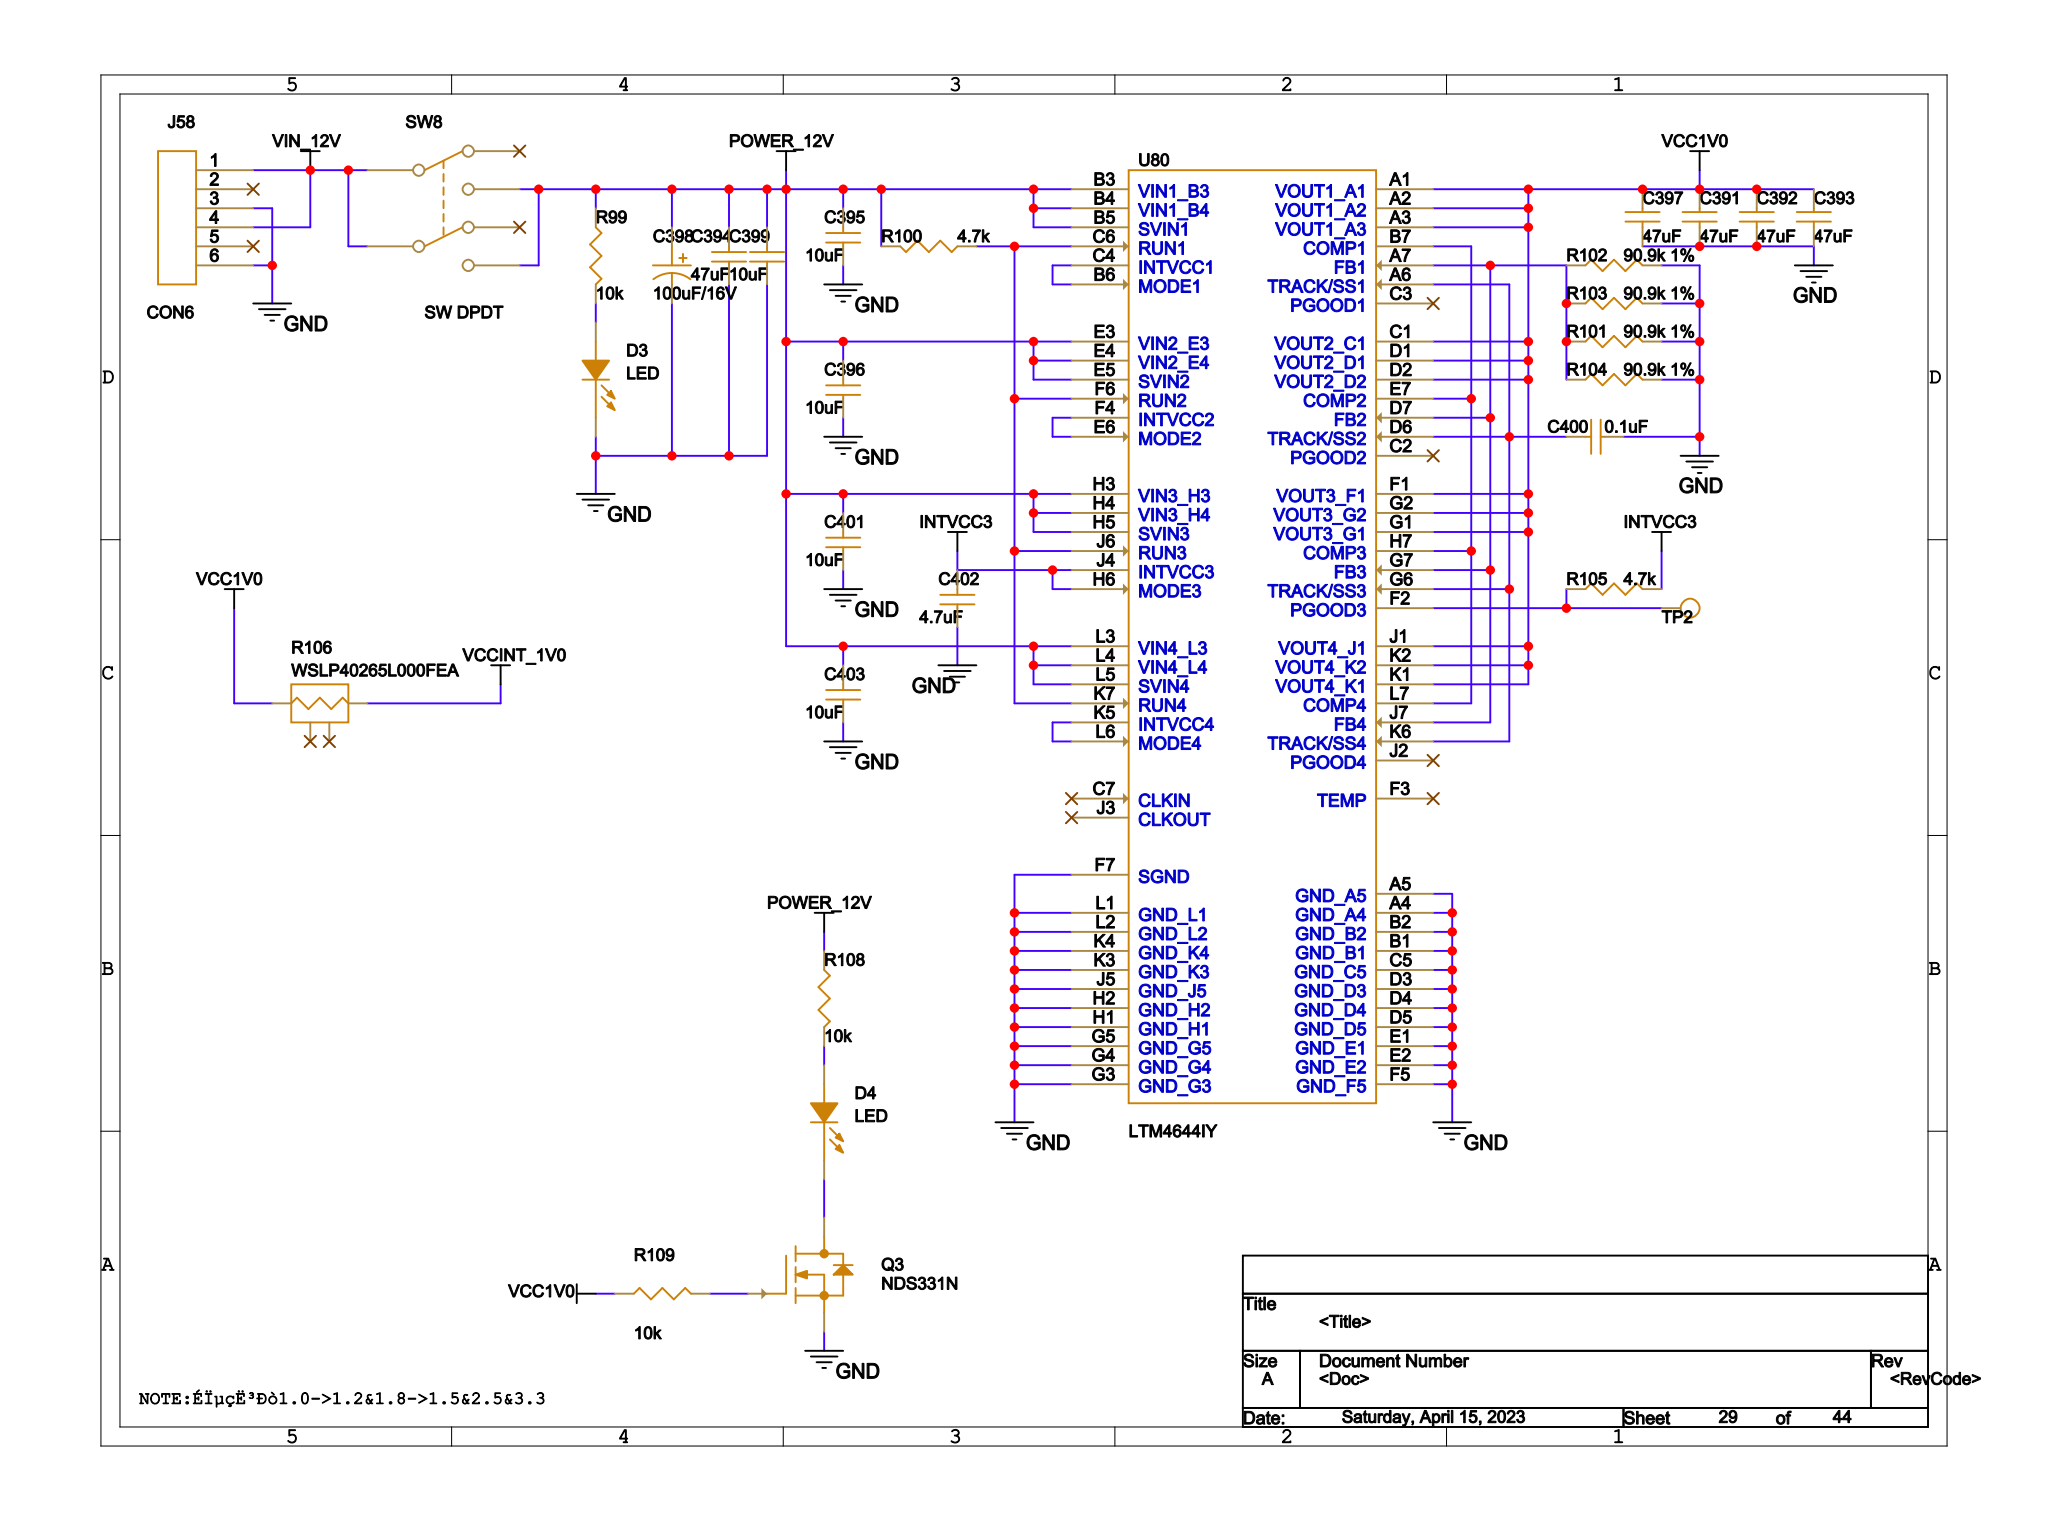Circuit board | Cadence Allegro | 1034 parts | 912 nets | one sheet of the schematic
Parts on this sheet (reference | value | footprint):
C391 | 47uF | C0402
C392 | 47uF | C0402
C393 | 47uF | C0402
C394 | 47uF | C0402
C395 | 10uF | C0402
C396 | 10uF | C0402
C397 | 47uF | C0402
C398 | 100uF/16V | C0402
C399 | 10uF | C0402
C400 | 0.1uF | C0402
C401 | 10uF | C0402
C402 | 4.7uF | C0402
C403 | 10uF | C0402
D3 | LED | LED_0603
D4 | LED | LED_0603
J58 | CON6 | CON_MOL_5569_6P
Q3 | NDS331N | MOS_SOT23
R99 | 10k | R0402
R100 | 4.7k | R0402
R101 | 90.9k 1% | R0402
R102 | 90.9k 1% | R0402
R103 | 90.9k 1% | R0402
R104 | 90.9k 1% | R0402
R105 | 4.7k | R0402
R106 | WSLP40265L000FEA | WSLP4026
R108 | 10k | R0402
R109 | 10k | R0402
SW8 | SW DPDT | SW_450_500
TP2 | T POINT R | SMD_M3
U80 | LTM4644IY | BGA77-1_27-15_0X9_0-H5_21
Nets of these parts (net: part-pin ...):
GND: C391-2 C392-2 C393-2 C394-1 C395-1 C396-1 C397-2 C398-2 C399-1 C400-1 C401-1 C402-1 C403-1 D3-1 J58-3 J58-6 Q3-2 R101-2 R102-2 R103-2 R104-2 U80-A4 U80-A5 U80-B1 U80-B2 U80-C5 U80-D3 U80-D4 U80-D5 U80-E1 U80-E2 U80-F5 U80-F7 U80-G3 U80-G4 U80-G5 U80-H1 U80-H2 U80-J5 U80-K3 U80-K4 U80-L1 U80-L2
VCCINT_1V0: R106-2
N386955: C400-2 U80-A6 U80-D6 U80-G6 U80-K6
POWER_12V: C394-2 C395-2 C396-2 C398-1 C399-2 C401-2 C403-2 R99-1 R100-2 R108-1 SW8-3 SW8-6 U80-B3 U80-B4 U80-B5 U80-E3 U80-E4 U80-E5 U80-H3 U80-H4 U80-H5 U80-L3 U80-L4 U80-L5
VCC1V0: C391-1 C392-1 C393-1 C397-1 R106-1 R109-1 U80-A1 U80-A2 U80-A3 U80-C1 U80-D1 U80-D2 U80-F1 U80-G1 U80-G2 U80-J1 U80-K1 U80-K2
INTVCC3: C402-2 R105-2 U80-H6 U80-J4
N385268: D3-2 R99-2
N395091: D4-2 R108-2
N395059: D4-1 Q3-3
VIN_12V: J58-1 J58-4 SW8-2 SW8-5
N395547: Q3-1 R109-2
N387512: R101-1 R102-1 R103-1 R104-1 U80-A7 U80-D7 U80-G7 U80-J7
N382631: R100-1 U80-C6 U80-F6 U80-J6 U80-K7
N392574: R105-1 TP2-1 U80-F2